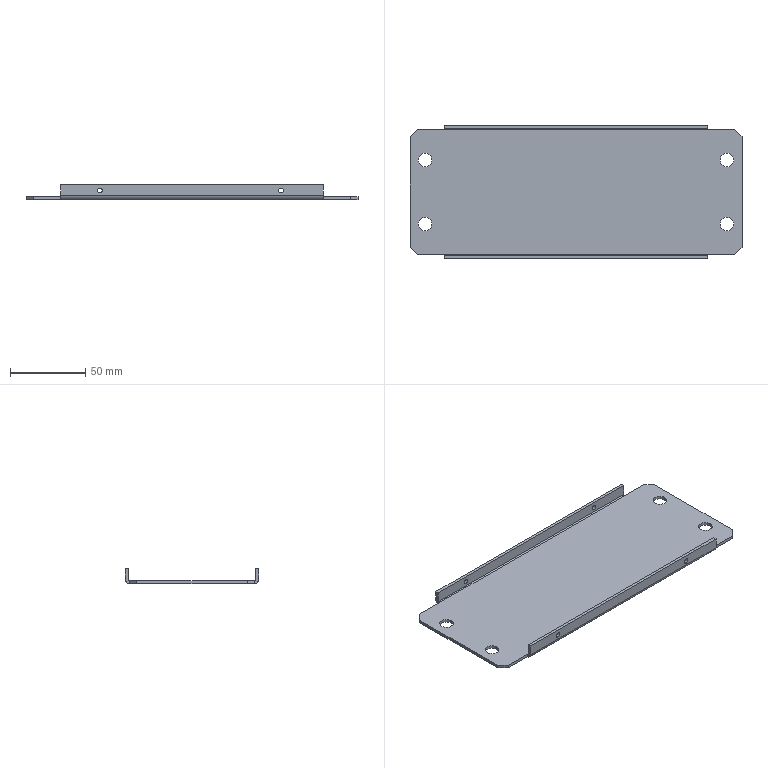Part | STEP file | Indicator plate | 1 solid | 42 faces | box 220 x 88.473 x 10.009 mm | volume 42803 mm3 | plane 22 | cylinder 20 | commonest cylinder face diameters 3.3 x8 9 x8 1.473 x2 5.473 x2